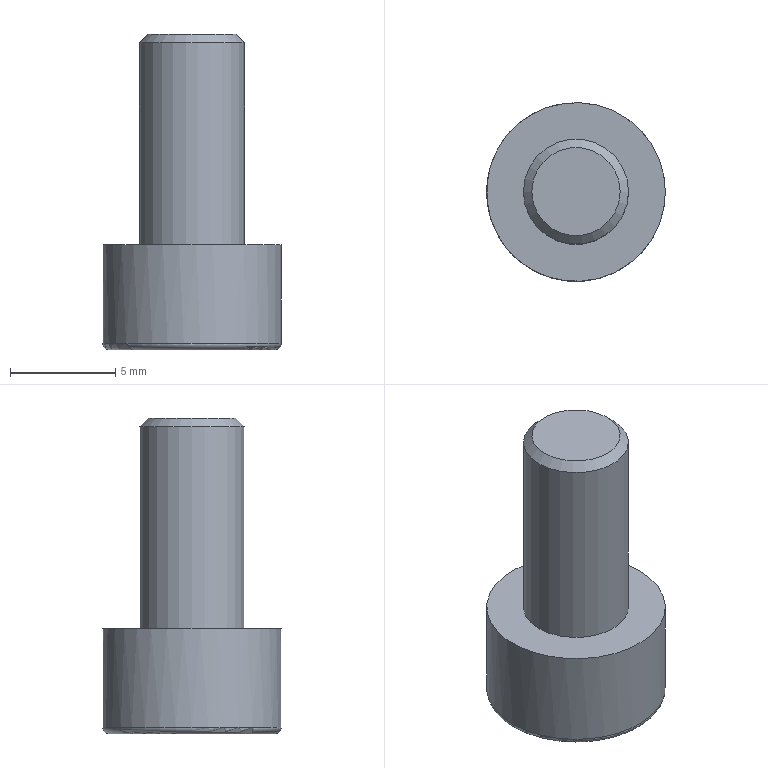Part | STEP file | 200 mesh_id86_xmt | 1 solid | 20 faces | box 8.5 x 8.5 x 15 mm | volume 436.532 mm3 | plane 10 | cylinder 8 | torus 1 | cone 1 | commonest cylinder face diameters 0.6 x6 5 x1 8.5 x1
STEP:
#1=CARTESIAN_POINT('',(-16904.349,-4062.769,92.258));
#2=VERTEX_POINT('',#1);
#3=CARTESIAN_POINT('',(-16906.849,-4062.769,92.258));
#4=DIRECTION('',(0.,0.,1.));
#5=DIRECTION('',(1.,0.,0.));
#6=AXIS2_PLACEMENT_3D('',#3,#4,#5);
#7=CIRCLE('',#6,2.5);
#8=EDGE_CURVE('',#2,#2,#7,.T.);
#9=ORIENTED_EDGE('',*,*,#8,.F.);
#10=EDGE_LOOP('',(#9));
#11=FACE_BOUND('',#10,.T.);
#12=CARTESIAN_POINT('',(-16902.599,-4062.769,92.258));
#13=VERTEX_POINT('',#12);
#14=CARTESIAN_POINT('',(-16906.849,-4062.769,92.258));
#15=DIRECTION('',(0.,0.,-1.));
#16=DIRECTION('',(1.,0.,0.));
#17=AXIS2_PLACEMENT_3D('',#14,#15,#16);
#18=CIRCLE('',#17,4.25);
#19=EDGE_CURVE('',#13,#13,#18,.T.);
#20=ORIENTED_EDGE('',*,*,#19,.F.);
#21=EDGE_LOOP('',(#20));
#22=FACE_BOUND('',#21,.T.);
#23=CARTESIAN_POINT('',(-16906.849,-4062.769,92.258));
#24=DIRECTION('',(0.,0.,1.));
#25=DIRECTION('',(1.,0.,0.));
#26=AXIS2_PLACEMENT_3D('',#23,#24,#25);
#27=PLANE('',#26);
#28=ADVANCED_FACE('',(#11,#22),#27,.T.);
#29=CARTESIAN_POINT('',(-16906.849,-4065.425,87.258));
#30=VERTEX_POINT('',#29);
#31=CARTESIAN_POINT('',(-16904.549,-4064.097,87.258));
#32=VERTEX_POINT('',#31);
#33=CARTESIAN_POINT('',(-16904.699,-4064.184,87.258));
#34=DIRECTION('',(0.866,0.5,0.));
#35=VECTOR('',#34,1.);
#36=LINE('',#33,#35);
#37=EDGE_CURVE('',#30,#32,#36,.T.);
#38=ORIENTED_EDGE('',*,*,#37,.T.);
#39=CARTESIAN_POINT('',(-16904.549,-4061.441,87.258));
#40=VERTEX_POINT('',#39);
#41=CARTESIAN_POINT('',(-16904.549,-4061.614,87.258));
#42=DIRECTION('',(0.,1.,0.));
#43=VECTOR('',#42,1.);
#44=LINE('',#41,#43);
#45=EDGE_CURVE('',#32,#40,#44,.T.);
#46=ORIENTED_EDGE('',*,*,#45,.T.);
#47=CARTESIAN_POINT('',(-16906.849,-4060.113,87.258));
#48=VERTEX_POINT('',#47);
#49=CARTESIAN_POINT('',(-16906.699,-4060.2,87.258));
#50=DIRECTION('',(-0.866,0.5,0.));
#51=VECTOR('',#50,1.);
#52=LINE('',#49,#51);
#53=EDGE_CURVE('',#40,#48,#52,.T.);
#54=ORIENTED_EDGE('',*,*,#53,.T.);
#55=CARTESIAN_POINT('',(-16909.149,-4061.441,87.258));
#56=VERTEX_POINT('',#55);
#57=CARTESIAN_POINT('',(-16908.999,-4061.355,87.258));
#58=DIRECTION('',(-0.866,-0.5,0.));
#59=VECTOR('',#58,1.);
#60=LINE('',#57,#59);
#61=EDGE_CURVE('',#48,#56,#60,.T.);
#62=ORIENTED_EDGE('',*,*,#61,.T.);
#63=CARTESIAN_POINT('',(-16909.149,-4064.097,87.258));
#64=VERTEX_POINT('',#63);
#65=CARTESIAN_POINT('',(-16909.149,-4063.924,87.258));
#66=DIRECTION('',(0.,-1.,0.));
#67=VECTOR('',#66,1.);
#68=LINE('',#65,#67);
#69=EDGE_CURVE('',#56,#64,#68,.T.);
#70=ORIENTED_EDGE('',*,*,#69,.T.);
#71=CARTESIAN_POINT('',(-16906.999,-4065.338,87.258));
#72=DIRECTION('',(0.866,-0.5,0.));
#73=VECTOR('',#72,1.);
#74=LINE('',#71,#73);
#75=EDGE_CURVE('',#64,#30,#74,.T.);
#76=ORIENTED_EDGE('',*,*,#75,.T.);
#77=EDGE_LOOP('',(#38,#46,#54,#62,#70,#76));
#78=FACE_BOUND('',#77,.T.);
#79=CARTESIAN_POINT('',(-16910.799,-4062.769,87.258));
#80=VERTEX_POINT('',#79);
#81=CARTESIAN_POINT('',(-16906.849,-4062.769,87.258));
#82=DIRECTION('',(0.,0.,-1.));
#83=DIRECTION('',(-1.,0.,0.));
#84=AXIS2_PLACEMENT_3D('',#81,#82,#83);
#85=CIRCLE('',#84,3.95);
#86=EDGE_CURVE('',#80,#80,#85,.T.);
#87=ORIENTED_EDGE('',*,*,#86,.T.);
#88=EDGE_LOOP('',(#87));
#89=FACE_BOUND('',#88,.T.);
#90=CARTESIAN_POINT('',(-16906.849,-4062.769,87.258));
#91=DIRECTION('',(0.,0.,-1.));
#92=DIRECTION('',(-1.,0.,0.));
#93=AXIS2_PLACEMENT_3D('',#90,#91,#92);
#94=PLANE('',#93);
#95=ADVANCED_FACE('',(#78,#89),#94,.T.);
#96=CARTESIAN_POINT('',(-16911.099,-4062.769,87.558));
#97=VERTEX_POINT('',#96);
#98=CARTESIAN_POINT('',(-16906.849,-4062.769,87.558));
#99=DIRECTION('',(0.,0.,1.));
#100=DIRECTION('',(-1.,0.,0.));
#101=AXIS2_PLACEMENT_3D('',#98,#99,#100);
#102=CIRCLE('',#101,4.25);
#103=EDGE_CURVE('',#97,#97,#102,.T.);
#104=ORIENTED_EDGE('',*,*,#103,.T.);
#105=EDGE_LOOP('',(#104));
#106=FACE_BOUND('',#105,.T.);
#107=ORIENTED_EDGE('',*,*,#19,.T.);
#108=EDGE_LOOP('',(#107));
#109=FACE_BOUND('',#108,.T.);
#110=CARTESIAN_POINT('',(-16906.849,-4062.769,92.258));
#111=DIRECTION('',(0.,0.,-1.));
#112=DIRECTION('',(1.,0.,0.));
#113=AXIS2_PLACEMENT_3D('',#110,#111,#112);
#114=CYLINDRICAL_SURFACE('',#113,4.25);
#115=ADVANCED_FACE('',(#106,#109),#114,.T.);
#116=ORIENTED_EDGE('',*,*,#86,.F.);
#117=EDGE_LOOP('',(#116));
#118=FACE_BOUND('',#117,.T.);
#119=ORIENTED_EDGE('',*,*,#103,.F.);
#120=EDGE_LOOP('',(#119));
#121=FACE_BOUND('',#120,.T.);
#122=CARTESIAN_POINT('',(-16906.849,-4062.769,87.558));
#123=DIRECTION('',(0.,0.,-1.));
#124=DIRECTION('',(-1.,0.,0.));
#125=AXIS2_PLACEMENT_3D('',#122,#123,#124);
#126=TOROIDAL_SURFACE('',#125,3.95,0.3);
#127=ADVANCED_FACE('',(#118,#121),#126,.T.);
#128=CARTESIAN_POINT('',(-16904.849,-4063.924,87.558));
#129=VERTEX_POINT('',#128);
#130=CARTESIAN_POINT('',(-16904.849,-4063.924,90.258));
#131=VERTEX_POINT('',#130);
#132=CARTESIAN_POINT('',(-16904.849,-4063.924,90.258));
#133=DIRECTION('',(0.,0.,1.));
#134=VECTOR('',#133,1.);
#135=LINE('',#132,#134);
#136=EDGE_CURVE('',#129,#131,#135,.T.);
#137=ORIENTED_EDGE('',*,*,#136,.F.);
#138=CARTESIAN_POINT('',(-16906.849,-4065.079,87.558));
#139=VERTEX_POINT('',#138);
#140=CARTESIAN_POINT('',(-16906.849,-4065.079,87.558));
#141=DIRECTION('',(-0.866,-0.5,0.));
#142=VECTOR('',#141,1.);
#143=LINE('',#140,#142);
#144=EDGE_CURVE('',#129,#139,#143,.T.);
#145=ORIENTED_EDGE('',*,*,#144,.T.);
#146=CARTESIAN_POINT('',(-16906.849,-4065.079,90.258));
#147=VERTEX_POINT('',#146);
#148=CARTESIAN_POINT('',(-16906.849,-4065.079,90.258));
#149=DIRECTION('',(0.,0.,1.));
#150=VECTOR('',#149,1.);
#151=LINE('',#148,#150);
#152=EDGE_CURVE('',#139,#147,#151,.T.);
#153=ORIENTED_EDGE('',*,*,#152,.T.);
#154=CARTESIAN_POINT('',(-16904.849,-4063.924,90.258));
#155=DIRECTION('',(0.866,0.5,0.));
#156=VECTOR('',#155,1.);
#157=LINE('',#154,#156);
#158=EDGE_CURVE('',#147,#131,#157,.T.);
#159=ORIENTED_EDGE('',*,*,#158,.T.);
#160=EDGE_LOOP('',(#137,#145,#153,#159));
#161=FACE_OUTER_BOUND('',#160,.T.);
#162=CARTESIAN_POINT('',(-16904.849,-4063.924,90.258));
#163=DIRECTION('',(0.5,-0.866,0.));
#164=DIRECTION('',(0.866,0.5,0.));
#165=AXIS2_PLACEMENT_3D('',#162,#163,#164);
#166=PLANE('',#165);
#167=ADVANCED_FACE('',(#161),#166,.F.);
#168=ORIENTED_EDGE('',*,*,#152,.F.);
#169=CARTESIAN_POINT('',(-16908.849,-4063.924,87.558));
#170=VERTEX_POINT('',#169);
#171=CARTESIAN_POINT('',(-16908.849,-4063.924,87.558));
#172=DIRECTION('',(-0.866,0.5,0.));
#173=VECTOR('',#172,1.);
#174=LINE('',#171,#173);
#175=EDGE_CURVE('',#139,#170,#174,.T.);
#176=ORIENTED_EDGE('',*,*,#175,.T.);
#177=CARTESIAN_POINT('',(-16908.849,-4063.924,90.258));
#178=VERTEX_POINT('',#177);
#179=CARTESIAN_POINT('',(-16908.849,-4063.924,90.258));
#180=DIRECTION('',(0.,0.,1.));
#181=VECTOR('',#180,1.);
#182=LINE('',#179,#181);
#183=EDGE_CURVE('',#170,#178,#182,.T.);
#184=ORIENTED_EDGE('',*,*,#183,.T.);
#185=CARTESIAN_POINT('',(-16906.849,-4065.079,90.258));
#186=DIRECTION('',(0.866,-0.5,0.));
#187=VECTOR('',#186,1.);
#188=LINE('',#185,#187);
#189=EDGE_CURVE('',#178,#147,#188,.T.);
#190=ORIENTED_EDGE('',*,*,#189,.T.);
#191=EDGE_LOOP('',(#168,#176,#184,#190));
#192=FACE_OUTER_BOUND('',#191,.T.);
#193=CARTESIAN_POINT('',(-16906.849,-4065.079,90.258));
#194=DIRECTION('',(-0.5,-0.866,0.));
#195=DIRECTION('',(0.866,-0.5,0.));
#196=AXIS2_PLACEMENT_3D('',#193,#194,#195);
#197=PLANE('',#196);
#198=ADVANCED_FACE('',(#192),#197,.F.);
#199=ORIENTED_EDGE('',*,*,#183,.F.);
#200=CARTESIAN_POINT('',(-16908.849,-4061.614,87.558));
#201=VERTEX_POINT('',#200);
#202=CARTESIAN_POINT('',(-16908.849,-4061.614,87.558));
#203=DIRECTION('',(0.,1.,0.));
#204=VECTOR('',#203,1.);
#205=LINE('',#202,#204);
#206=EDGE_CURVE('',#170,#201,#205,.T.);
#207=ORIENTED_EDGE('',*,*,#206,.T.);
#208=CARTESIAN_POINT('',(-16908.849,-4061.614,90.258));
#209=VERTEX_POINT('',#208);
#210=CARTESIAN_POINT('',(-16908.849,-4061.614,90.258));
#211=DIRECTION('',(0.,0.,1.));
#212=VECTOR('',#211,1.);
#213=LINE('',#210,#212);
#214=EDGE_CURVE('',#201,#209,#213,.T.);
#215=ORIENTED_EDGE('',*,*,#214,.T.);
#216=CARTESIAN_POINT('',(-16908.849,-4063.924,90.258));
#217=DIRECTION('',(0.,-1.,0.));
#218=VECTOR('',#217,1.);
#219=LINE('',#216,#218);
#220=EDGE_CURVE('',#209,#178,#219,.T.);
#221=ORIENTED_EDGE('',*,*,#220,.T.);
#222=EDGE_LOOP('',(#199,#207,#215,#221));
#223=FACE_OUTER_BOUND('',#222,.T.);
#224=CARTESIAN_POINT('',(-16908.849,-4063.924,90.258));
#225=DIRECTION('',(-1.,0.,0.));
#226=DIRECTION('',(0.,0.,1.));
#227=AXIS2_PLACEMENT_3D('',#224,#225,#226);
#228=PLANE('',#227);
#229=ADVANCED_FACE('',(#223),#228,.F.);
#230=ORIENTED_EDGE('',*,*,#214,.F.);
#231=CARTESIAN_POINT('',(-16906.849,-4060.46,87.558));
#232=VERTEX_POINT('',#231);
#233=CARTESIAN_POINT('',(-16906.849,-4060.46,87.558));
#234=DIRECTION('',(0.866,0.5,0.));
#235=VECTOR('',#234,1.);
#236=LINE('',#233,#235);
#237=EDGE_CURVE('',#201,#232,#236,.T.);
#238=ORIENTED_EDGE('',*,*,#237,.T.);
#239=CARTESIAN_POINT('',(-16906.849,-4060.46,90.258));
#240=VERTEX_POINT('',#239);
#241=CARTESIAN_POINT('',(-16906.849,-4060.46,90.258));
#242=DIRECTION('',(0.,0.,1.));
#243=VECTOR('',#242,1.);
#244=LINE('',#241,#243);
#245=EDGE_CURVE('',#232,#240,#244,.T.);
#246=ORIENTED_EDGE('',*,*,#245,.T.);
#247=CARTESIAN_POINT('',(-16908.849,-4061.614,90.258));
#248=DIRECTION('',(-0.866,-0.5,0.));
#249=VECTOR('',#248,1.);
#250=LINE('',#247,#249);
#251=EDGE_CURVE('',#240,#209,#250,.T.);
#252=ORIENTED_EDGE('',*,*,#251,.T.);
#253=EDGE_LOOP('',(#230,#238,#246,#252));
#254=FACE_OUTER_BOUND('',#253,.T.);
#255=CARTESIAN_POINT('',(-16908.849,-4061.614,90.258));
#256=DIRECTION('',(-0.5,0.866,0.));
#257=DIRECTION('',(-0.866,-0.5,0.));
#258=AXIS2_PLACEMENT_3D('',#255,#256,#257);
#259=PLANE('',#258);
#260=ADVANCED_FACE('',(#254),#259,.F.);
#261=ORIENTED_EDGE('',*,*,#245,.F.);
#262=CARTESIAN_POINT('',(-16904.849,-4061.614,87.558));
#263=VERTEX_POINT('',#262);
#264=CARTESIAN_POINT('',(-16904.849,-4061.614,87.558));
#265=DIRECTION('',(0.866,-0.5,0.));
#266=VECTOR('',#265,1.);
#267=LINE('',#264,#266);
#268=EDGE_CURVE('',#232,#263,#267,.T.);
#269=ORIENTED_EDGE('',*,*,#268,.T.);
#270=CARTESIAN_POINT('',(-16904.849,-4061.614,90.258));
#271=VERTEX_POINT('',#270);
#272=CARTESIAN_POINT('',(-16904.849,-4061.614,90.258));
#273=DIRECTION('',(0.,0.,1.));
#274=VECTOR('',#273,1.);
#275=LINE('',#272,#274);
#276=EDGE_CURVE('',#263,#271,#275,.T.);
#277=ORIENTED_EDGE('',*,*,#276,.T.);
#278=CARTESIAN_POINT('',(-16906.849,-4060.46,90.258));
#279=DIRECTION('',(-0.866,0.5,0.));
#280=VECTOR('',#279,1.);
#281=LINE('',#278,#280);
#282=EDGE_CURVE('',#271,#240,#281,.T.);
#283=ORIENTED_EDGE('',*,*,#282,.T.);
#284=EDGE_LOOP('',(#261,#269,#277,#283));
#285=FACE_OUTER_BOUND('',#284,.T.);
#286=CARTESIAN_POINT('',(-16906.849,-4060.46,90.258));
#287=DIRECTION('',(0.5,0.866,0.));
#288=DIRECTION('',(-0.866,0.5,0.));
#289=AXIS2_PLACEMENT_3D('',#286,#287,#288);
#290=PLANE('',#289);
#291=ADVANCED_FACE('',(#285),#290,.F.);
#292=ORIENTED_EDGE('',*,*,#276,.F.);
#293=CARTESIAN_POINT('',(-16904.849,-4063.924,87.558));
#294=DIRECTION('',(0.,-1.,0.));
#295=VECTOR('',#294,1.);
#296=LINE('',#293,#295);
#297=EDGE_CURVE('',#263,#129,#296,.T.);
#298=ORIENTED_EDGE('',*,*,#297,.T.);
#299=ORIENTED_EDGE('',*,*,#136,.T.);
#300=CARTESIAN_POINT('',(-16904.849,-4061.614,90.258));
#301=DIRECTION('',(0.,1.,0.));
#302=VECTOR('',#301,1.);
#303=LINE('',#300,#302);
#304=EDGE_CURVE('',#131,#271,#303,.T.);
#305=ORIENTED_EDGE('',*,*,#304,.T.);
#306=EDGE_LOOP('',(#292,#298,#299,#305));
#307=FACE_OUTER_BOUND('',#306,.T.);
#308=CARTESIAN_POINT('',(-16904.849,-4061.614,90.258));
#309=DIRECTION('',(1.,0.,0.));
#310=DIRECTION('',(0.,0.,-1.));
#311=AXIS2_PLACEMENT_3D('',#308,#309,#310);
#312=PLANE('',#311);
#313=ADVANCED_FACE('',(#307),#312,.F.);
#314=ORIENTED_EDGE('',*,*,#158,.F.);
#315=ORIENTED_EDGE('',*,*,#189,.F.);
#316=ORIENTED_EDGE('',*,*,#220,.F.);
#317=ORIENTED_EDGE('',*,*,#251,.F.);
#318=ORIENTED_EDGE('',*,*,#282,.F.);
#319=ORIENTED_EDGE('',*,*,#304,.F.);
#320=EDGE_LOOP('',(#314,#315,#316,#317,#318,#319));
#321=FACE_OUTER_BOUND('',#320,.T.);
#322=CARTESIAN_POINT('',(0.,0.,90.258));
#323=DIRECTION('',(0.,0.,-1.));
#324=DIRECTION('',(-1.,0.,0.));
#325=AXIS2_PLACEMENT_3D('',#322,#323,#324);
#326=PLANE('',#325);
#327=ADVANCED_FACE('',(#321),#326,.T.);
#328=CARTESIAN_POINT('',(-16909.149,-4064.097,87.558));
#329=DIRECTION('',(0.5,-0.866,0.));
#330=DIRECTION('',(-0.866,-0.5,0.));
#331=AXIS2_PLACEMENT_3D('',#328,#329,#330);
#332=ELLIPSE('',#331,0.3464,0.3);
#333=EDGE_CURVE('',#64,#170,#332,.T.);
#334=ORIENTED_EDGE('',*,*,#333,.F.);
#335=ORIENTED_EDGE('',*,*,#69,.F.);
#336=CARTESIAN_POINT('',(-16909.149,-4061.441,87.558));
#337=DIRECTION('',(0.5,0.866,0.));
#338=DIRECTION('',(-0.866,0.5,0.));
#339=AXIS2_PLACEMENT_3D('',#336,#337,#338);
#340=ELLIPSE('',#339,0.3464,0.3);
#341=EDGE_CURVE('',#201,#56,#340,.T.);
#342=ORIENTED_EDGE('',*,*,#341,.F.);
#343=ORIENTED_EDGE('',*,*,#206,.F.);
#344=EDGE_LOOP('',(#334,#335,#342,#343));
#345=FACE_OUTER_BOUND('',#344,.T.);
#346=CARTESIAN_POINT('',(-16909.149,-4063.924,87.558));
#347=DIRECTION('',(0.,-1.,0.));
#348=DIRECTION('',(0.,0.,-1.));
#349=AXIS2_PLACEMENT_3D('',#346,#347,#348);
#350=CYLINDRICAL_SURFACE('',#349,0.3);
#351=ADVANCED_FACE('',(#345),#350,.T.);
#352=ORIENTED_EDGE('',*,*,#341,.T.);
#353=ORIENTED_EDGE('',*,*,#61,.F.);
#354=CARTESIAN_POINT('',(-16906.849,-4060.113,87.558));
#355=DIRECTION('',(1.,0.,0.));
#356=DIRECTION('',(0.,1.,0.));
#357=AXIS2_PLACEMENT_3D('',#354,#355,#356);
#358=ELLIPSE('',#357,0.3464,0.3);
#359=EDGE_CURVE('',#232,#48,#358,.T.);
#360=ORIENTED_EDGE('',*,*,#359,.F.);
#361=ORIENTED_EDGE('',*,*,#237,.F.);
#362=EDGE_LOOP('',(#352,#353,#360,#361));
#363=FACE_OUTER_BOUND('',#362,.T.);
#364=CARTESIAN_POINT('',(-16908.999,-4061.355,87.558));
#365=DIRECTION('',(-0.866,-0.5,0.));
#366=DIRECTION('',(0.5,-0.866,0.));
#367=AXIS2_PLACEMENT_3D('',#364,#365,#366);
#368=CYLINDRICAL_SURFACE('',#367,0.3);
#369=ADVANCED_FACE('',(#363),#368,.T.);
#370=ORIENTED_EDGE('',*,*,#333,.T.);
#371=ORIENTED_EDGE('',*,*,#175,.F.);
#372=CARTESIAN_POINT('',(-16906.849,-4065.425,87.558));
#373=DIRECTION('',(1.,0.,0.));
#374=DIRECTION('',(0.,-1.,0.));
#375=AXIS2_PLACEMENT_3D('',#372,#373,#374);
#376=ELLIPSE('',#375,0.3464,0.3);
#377=EDGE_CURVE('',#30,#139,#376,.T.);
#378=ORIENTED_EDGE('',*,*,#377,.F.);
#379=ORIENTED_EDGE('',*,*,#75,.F.);
#380=EDGE_LOOP('',(#370,#371,#378,#379));
#381=FACE_OUTER_BOUND('',#380,.T.);
#382=CARTESIAN_POINT('',(-16906.999,-4065.338,87.558));
#383=DIRECTION('',(0.866,-0.5,0.));
#384=DIRECTION('',(0.5,0.866,0.));
#385=AXIS2_PLACEMENT_3D('',#382,#383,#384);
#386=CYLINDRICAL_SURFACE('',#385,0.3);
#387=ADVANCED_FACE('',(#381),#386,.T.);
#388=ORIENTED_EDGE('',*,*,#359,.T.);
#389=ORIENTED_EDGE('',*,*,#53,.F.);
#390=CARTESIAN_POINT('',(-16904.549,-4061.441,87.558));
#391=DIRECTION('',(0.5,-0.866,0.));
#392=DIRECTION('',(0.866,0.5,0.));
#393=AXIS2_PLACEMENT_3D('',#390,#391,#392);
#394=ELLIPSE('',#393,0.3464,0.3);
#395=EDGE_CURVE('',#263,#40,#394,.T.);
#396=ORIENTED_EDGE('',*,*,#395,.F.);
#397=ORIENTED_EDGE('',*,*,#268,.F.);
#398=EDGE_LOOP('',(#388,#389,#396,#397));
#399=FACE_OUTER_BOUND('',#398,.T.);
#400=CARTESIAN_POINT('',(-16906.699,-4060.2,87.558));
#401=DIRECTION('',(-0.866,0.5,0.));
#402=DIRECTION('',(-0.5,-0.866,0.));
#403=AXIS2_PLACEMENT_3D('',#400,#401,#402);
#404=CYLINDRICAL_SURFACE('',#403,0.3);
#405=ADVANCED_FACE('',(#399),#404,.T.);
#406=ORIENTED_EDGE('',*,*,#377,.T.);
#407=ORIENTED_EDGE('',*,*,#144,.F.);
#408=CARTESIAN_POINT('',(-16904.549,-4064.097,87.558));
#409=DIRECTION('',(0.5,0.866,0.));
#410=DIRECTION('',(-0.866,0.5,0.));
#411=AXIS2_PLACEMENT_3D('',#408,#409,#410);
#412=ELLIPSE('',#411,0.3464,0.3);
#413=EDGE_CURVE('',#32,#129,#412,.T.);
#414=ORIENTED_EDGE('',*,*,#413,.F.);
#415=ORIENTED_EDGE('',*,*,#37,.F.);
#416=EDGE_LOOP('',(#406,#407,#414,#415));
#417=FACE_OUTER_BOUND('',#416,.T.);
#418=CARTESIAN_POINT('',(-16904.699,-4064.184,87.558));
#419=DIRECTION('',(0.866,0.5,0.));
#420=DIRECTION('',(-0.5,0.866,0.));
#421=AXIS2_PLACEMENT_3D('',#418,#419,#420);
#422=CYLINDRICAL_SURFACE('',#421,0.3);
#423=ADVANCED_FACE('',(#417),#422,.T.);
#424=ORIENTED_EDGE('',*,*,#395,.T.);
#425=ORIENTED_EDGE('',*,*,#45,.F.);
#426=ORIENTED_EDGE('',*,*,#413,.T.);
#427=ORIENTED_EDGE('',*,*,#297,.F.);
#428=EDGE_LOOP('',(#424,#425,#426,#427));
#429=FACE_OUTER_BOUND('',#428,.T.);
#430=CARTESIAN_POINT('',(-16904.549,-4061.614,87.558));
#431=DIRECTION('',(0.,1.,0.));
#432=DIRECTION('',(0.,0.,1.));
#433=AXIS2_PLACEMENT_3D('',#430,#431,#432);
#434=CYLINDRICAL_SURFACE('',#433,0.3);
#435=ADVANCED_FACE('',(#429),#434,.T.);
#436=CARTESIAN_POINT('',(-16904.349,-4062.769,101.858));
#437=VERTEX_POINT('',#436);
#438=CARTESIAN_POINT('',(-16906.849,-4062.769,101.858));
#439=DIRECTION('',(0.,0.,-1.));
#440=DIRECTION('',(1.,0.,0.));
#441=AXIS2_PLACEMENT_3D('',#438,#439,#440);
#442=CIRCLE('',#441,2.5);
#443=EDGE_CURVE('',#437,#437,#442,.T.);
#444=ORIENTED_EDGE('',*,*,#443,.T.);
#445=EDGE_LOOP('',(#444));
#446=FACE_BOUND('',#445,.T.);
#447=ORIENTED_EDGE('',*,*,#8,.T.);
#448=EDGE_LOOP('',(#447));
#449=FACE_BOUND('',#448,.T.);
#450=CARTESIAN_POINT('',(-16906.849,-4062.769,92.258));
#451=DIRECTION('',(0.,0.,1.));
#452=DIRECTION('',(1.,0.,0.));
#453=AXIS2_PLACEMENT_3D('',#450,#451,#452);
#454=CYLINDRICAL_SURFACE('',#453,2.5);
#455=ADVANCED_FACE('',(#446,#449),#454,.T.);
#456=CARTESIAN_POINT('',(-16904.749,-4062.769,102.258));
#457=VERTEX_POINT('',#456);
#458=CARTESIAN_POINT('',(-16906.849,-4062.769,102.258));
#459=DIRECTION('',(0.,0.,1.));
#460=DIRECTION('',(1.,0.,0.));
#461=AXIS2_PLACEMENT_3D('',#458,#459,#460);
#462=CIRCLE('',#461,2.1);
#463=EDGE_CURVE('',#457,#457,#462,.T.);
#464=ORIENTED_EDGE('',*,*,#463,.T.);
#465=EDGE_LOOP('',(#464));
#466=FACE_OUTER_BOUND('',#465,.T.);
#467=CARTESIAN_POINT('',(-16906.849,-4062.769,102.258));
#468=DIRECTION('',(0.,0.,1.));
#469=DIRECTION('',(1.,0.,0.));
#470=AXIS2_PLACEMENT_3D('',#467,#468,#469);
#471=PLANE('',#470);
#472=ADVANCED_FACE('',(#466),#471,.T.);
#473=ORIENTED_EDGE('',*,*,#463,.F.);
#474=EDGE_LOOP('',(#473));
#475=FACE_BOUND('',#474,.T.);
#476=ORIENTED_EDGE('',*,*,#443,.F.);
#477=EDGE_LOOP('',(#476));
#478=FACE_BOUND('',#477,.T.);
#479=CARTESIAN_POINT('',(-16906.849,-4062.769,101.858));
#480=DIRECTION('',(0.,0.,-1.));
#481=DIRECTION('',(-1.,0.,0.));
#482=AXIS2_PLACEMENT_3D('',#479,#480,#481);
#483=CONICAL_SURFACE('',#482,2.5,45.);
#484=ADVANCED_FACE('',(#475,#478),#483,.T.);
#485=CLOSED_SHELL('',(#28,#95,#115,#127,#167,#198,#229,#260,#291,#313,#327,#351,#369,#387,#405,#423,#435,#455,#472,#484));
#486=MANIFOLD_SOLID_BREP('',#485);
#487=(LENGTH_UNIT()NAMED_UNIT(*)SI_UNIT(.MILLI.,.METRE.));
#488=UNCERTAINTY_MEASURE_WITH_UNIT(LENGTH_MEASURE(0.00002),#487,'','');
#489=(NAMED_UNIT(*)PLANE_ANGLE_UNIT()SI_UNIT($,.RADIAN.));
#490=PLANE_ANGLE_MEASURE_WITH_UNIT(PLANE_ANGLE_MEASURE(0.01745),#489);
#491=DIMENSIONAL_EXPONENTS(0.,0.,0.,0.,0.,0.,0.);
#492=(CONVERSION_BASED_UNIT('DEGREE',#490)NAMED_UNIT(#491)PLANE_ANGLE_UNIT());
#493=(NAMED_UNIT(*)SI_UNIT($,.STERADIAN.)SOLID_ANGLE_UNIT());
#494=(GEOMETRIC_REPRESENTATION_CONTEXT(3)GLOBAL_UNCERTAINTY_ASSIGNED_CONTEXT((#488))GLOBAL_UNIT_ASSIGNED_CONTEXT((#487,#492,#493))REPRESENTATION_CONTEXT('',''));
#495=ADVANCED_BREP_SHAPE_REPRESENTATION('',(#486),#494);